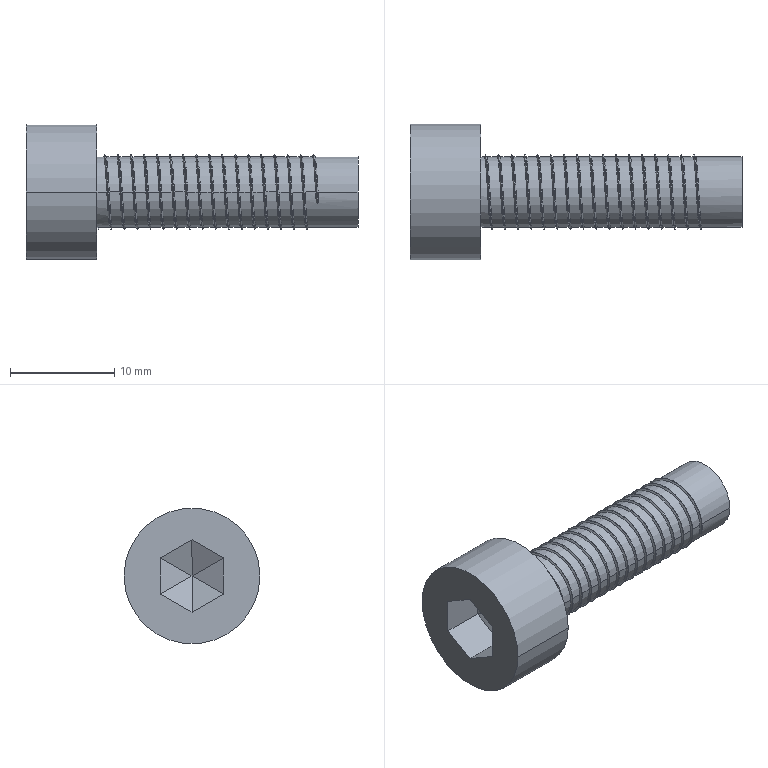Part | SolidWorks | features BlendCut 1, ICE 1, Revolution 1, SweepThread 1 | 1 solid | 58 faces | box 31.8 x 13 x 13 mm | volume 1679 mm3 | cylinder 38 | plane 17 | spline 3 | commonest cylinder face diameters 6.8 x36 13 x2